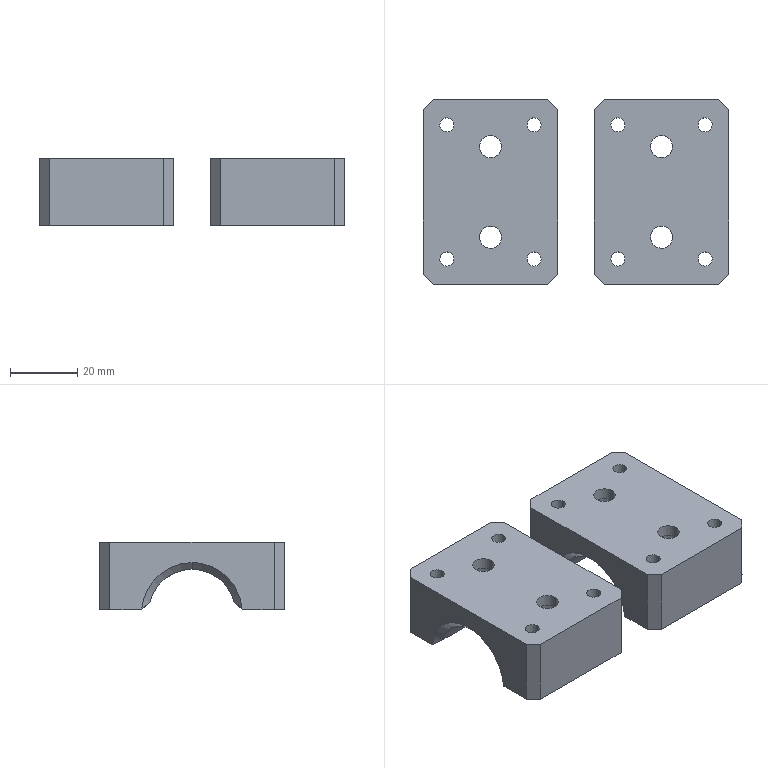NC program | NX | posted with a generic post | part box 91 x 55 x 20 mm
Lines 4306 to 5121 of 95737:
(FIXED_CONTOUR , TOOL : R3)
N8562 T17 M6
N8564 G54
N8566 G17 G0 G90 X3.472 Y-12.781 S9500 M3
N8568 G43 Z30. H17
N8570 Z2.4
N8572 G94 G1 Z-2.825 F1000.
N8574 X3.459 Y-12.768 Z-2.953 F3000.
N8576 X3.448 Y-12.757 Z-3.126
N8578 X3.439 Y-12.747 Z-3.346
N8580 X3.43 Y-12.738 Z-3.478
N8582 X3.419 Y-12.727 Z-3.695
N8584 X3.394 Y-12.702 Z-3.972
N8586 X3.383 Y-12.692 Z-4.138
N8588 X3.386 Y-12.662 Z-4.327
N8590 X3.385 Y-12.623 Z-4.543
N8592 X3.387 Y-12.596 Z-4.676
N8594 Y-12.576 Z-4.761
N8596 X3.397 Y-12.586 Z-4.673
N8598 X3.423 Y-12.613 Z-4.381
N8600 X3.44 Y-12.629 Z-4.127
N8602 X3.474 Y-12.664 Z-3.74
N8604 X3.483 Y-12.673 Z-3.565
N8606 X3.496 Y-12.686 Z-3.375
N8608 X3.504 Y-12.693 Z-3.202
N8610 X3.519 Y-12.708 Z-2.965
N8612 X3.535 Y-12.724 Z-2.813
N8614 X3.546 Y-12.735 Z-2.689
N8616 X3.575 Y-12.72 Z-2.638
N8618 X3.626 Y-12.697 Z-2.555
N8620 X3.609 Y-12.679 Z-2.674
N8622 X3.6 Y-12.671 Z-2.774
N8624 X3.578 Y-12.648 Z-2.991
N8626 X3.559 Y-12.63 Z-3.278
N8628 X3.554 Y-12.624 Z-3.404
N8630 X3.537 Y-12.607 Z-3.652
N8632 X3.53 Y-12.6 Z-3.785
N8634 X3.486 Y-12.556 Z-4.282
N8636 X3.475 Y-12.545 Z-4.455
N8638 X3.457 Y-12.527 Z-4.654
N8640 X3.396 Y-12.466 Z-5.176
N8642 X3.382 Y-12.453 Z-5.272
N8644 X3.381 Y-12.401 Z-5.46
N8646 X3.421 Y-12.441 Z-5.166
N8648 X3.482 Y-12.502 Z-4.646
N8650 X3.496 Y-12.516 Z-4.486
N8652 X3.505 Y-12.525 Z-4.348
N8654 X3.554 Y-12.574 Z-3.804
N8656 X3.56 Y-12.58 Z-3.689
N8658 X3.578 Y-12.598 Z-3.416
N8660 X3.583 Y-12.603 Z-3.31
N8662 X3.604 Y-12.624 Z-2.981
N8664 X3.628 Y-12.648 Z-2.757
N8666 X3.634 Y-12.654 Z-2.683
N8668 X3.661 Y-12.681 Z-2.499
N8670 X3.697 Y-12.667 Z-2.442
N8672 X3.659 Y-12.629 Z-2.693
N8674 X3.629 Y-12.598 Z-2.995
N8676 X3.606 Y-12.576 Z-3.343
N8678 X3.602 Y-12.572 Z-3.428
N8680 X3.582 Y-12.552 Z-3.726
N8682 X3.577 Y-12.547 Z-3.823
N8684 X3.525 Y-12.495 Z-4.413
N8686 X3.518 Y-12.488 Z-4.518
N8688 X3.507 Y-12.477 Z-4.638
N8690 X3.446 Y-12.416 Z-5.157
N8692 X3.379 Y-12.349 Z-5.647
N8694 X3.377 Y-12.297 Z-5.805
N8696 X3.41 Y-12.33 Z-5.607
N8698 X3.471 Y-12.391 Z-5.149
N8700 X3.532 Y-12.452 Z-4.63
N8702 X3.54 Y-12.459 Z-4.549
N8704 X3.544 Y-12.464 Z-4.479
N8706 X3.601 Y-12.52 Z-3.842
N8708 X3.605 Y-12.524 Z-3.763
N8710 X3.627 Y-12.546 Z-3.44
N8712 X3.63 Y-12.549 Z-3.375
N8714 X3.654 Y-12.574 Z-2.991
N8716 X3.685 Y-12.604 Z-2.702
N8718 X3.714 Y-12.633 Z-2.503
N8720 X3.736 Y-12.655 Z-2.387
N8722 X3.777 Y-12.645 Z-2.329
N8724 X3.751 Y-12.618 Z-2.459
N8726 X3.737 Y-12.604 Z-2.543
N8728 X3.711 Y-12.578 Z-2.713
N8730 X3.681 Y-12.548 Z-2.996
N8732 X3.652 Y-12.519 Z-3.453
N8734 X3.625 Y-12.492 Z-3.862
N8736 X3.559 Y-12.426 Z-4.622
N8738 X3.498 Y-12.365 Z-5.144
N8740 X3.437 Y-12.304 Z-5.602
N8742 X3.423 Y-12.29 Z-5.693
N8744 X3.377 Y-12.244 Z-5.964
N8746 Y-12.19 Z-6.129
N8748 X3.389 Y-12.202 Z-6.046
N8750 X3.446 Y-12.259 Z-5.714
N8752 X3.464 Y-12.276 Z-5.597
N8754 X3.525 Y-12.337 Z-5.139
N8756 X3.586 Y-12.398 Z-4.613
N8758 X3.651 Y-12.463 Z-3.883
N8760 X3.708 Y-12.52 Z-3.002
N8762 X3.738 Y-12.551 Z-2.728
N8764 X3.769 Y-12.581 Z-2.53
N8766 X3.777 Y-12.59 Z-2.483
N8768 X3.813 Y-12.625 Z-2.31
N8770 X3.822 Y-12.635 Z-2.269
N8772 X3.87 Y-12.626 Z-2.206
N8774 X3.845 Y-12.601 Z-2.31
N8776 X3.804 Y-12.56 Z-2.509
N8778 X3.784 Y-12.54 Z-2.628
N8780 X3.767 Y-12.523 Z-2.744
N8782 X3.736 Y-12.492 Z-3.012
N8784 X3.677 Y-12.433 Z-3.904
N8786 X3.614 Y-12.37 Z-4.609
N8788 X3.553 Y-12.309 Z-5.134
N8790 X3.492 Y-12.248 Z-5.592
N8792 X3.471 Y-12.226 Z-5.735
N8794 X3.401 Y-12.156 Z-6.144
N8796 X3.378 Y-12.133 Z-6.301
N8798 Y-12.098 Z-6.41
N8800 X3.38 Y-12.073 Z-6.478
N8802 X3.413 Y-12.106 Z-6.252
N8804 X3.498 Y-12.19 Z-5.759
N8806 X3.524 Y-12.217 Z-5.587
N8808 X3.585 Y-12.278 Z-5.128
N8810 X3.646 Y-12.339 Z-4.605
N8812 X3.707 Y-12.4 Z-3.928
N8814 X3.768 Y-12.461 Z-3.023
N8816 X3.78 Y-12.473 Z-2.926
N8818 X3.799 Y-12.491 Z-2.762
N8820 X3.835 Y-12.527 Z-2.537
N8822 X3.881 Y-12.574 Z-2.31
N8824 X3.924 Y-12.616 Z-2.136
N8826 X3.956 Y-12.611 Z-2.096
N8828 X3.987 Y-12.609 Z-2.06
N8830 X3.961 Y-12.583 Z-2.152
N8832 X3.919 Y-12.541 Z-2.326
N8834 X3.864 Y-12.487 Z-2.591
N8836 X3.834 Y-12.456 Z-2.782
N8838 X3.823 Y-12.445 Z-2.883
N8840 X3.803 Y-12.426 Z-3.035
N8842 X3.742 Y-12.365 Z-3.924
N8844 X3.681 Y-12.304 Z-4.6
N8846 X3.62 Y-12.243 Z-5.122
N8848 X3.559 Y-12.182 Z-5.581
N8850 X3.528 Y-12.15 Z-5.786
N8852 X3.427 Y-12.05 Z-6.373
N8854 X3.405 Y-12.027 Z-6.528
N8856 X3.383 Y-12.006 Z-6.656
N8858 X3.384 Y-11.991 Z-6.694
N8860 X3.381 Y-11.934 Z-6.833
N8862 X3.411 Y-11.964 Z-6.684
N8864 X3.428 Y-11.981 Z-6.585
N8866 X3.442 Y-11.994 Z-6.493
N8868 X3.558 Y-12.111 Z-5.813
N8870 X3.594 Y-12.147 Z-5.575
N8872 X3.655 Y-12.208 Z-5.116
N8874 X3.716 Y-12.269 Z-4.595
N8876 X3.777 Y-12.33 Z-3.92
N8878 X3.838 Y-12.391 Z-3.048
N8880 X3.872 Y-12.424 Z-2.782
N8882 X3.902 Y-12.454 Z-2.6
N8884 X3.96 Y-12.513 Z-2.318
N8886 X4.01 Y-12.562 Z-2.125
N8888 X4.054 Y-12.606 Z-1.983
N8890 X4.122 Y-12.605 Z-1.907
N8892 X4.091 Y-12.574 Z-1.999
N8894 X4.042 Y-12.525 Z-2.162
N8896 X3.995 Y-12.478 Z-2.342
N8898 X3.935 Y-12.418 Z-2.631
N8900 X3.899 Y-12.382 Z-2.856
N8902 X3.873 Y-12.356 Z-3.061
N8904 X3.865 Y-12.347 Z-3.165
N8906 X3.812 Y-12.295 Z-3.917
N8908 X3.751 Y-12.234 Z-4.59
N8910 X3.69 Y-12.173 Z-5.11
N8912 X3.629 Y-12.112 Z-5.568
N8914 X3.588 Y-12.071 Z-5.839
N8916 X3.446 Y-11.929 Z-6.671
N8918 X3.38 Y-11.862 Z-7.01
N8920 X3.378 Y-11.784 Z-7.181
N8922 X3.412 Y-11.818 Z-7.032
N8924 X3.485 Y-11.891 Z-6.661
N8926 X3.621 Y-12.027 Z-5.868
N8928 X3.668 Y-12.074 Z-5.562
N8930 X3.736 Y-12.142 Z-5.041
N8932 X3.79 Y-12.196 Z-4.585
N8934 X3.851 Y-12.257 Z-3.912
N8936 X3.895 Y-12.301 Z-3.269
N8938 X3.912 Y-12.318 Z-3.076
N8940 X3.942 Y-12.348 Z-2.842
N8942 X3.973 Y-12.379 Z-2.659
N8944 X4.034 Y-12.44 Z-2.369
N8946 X4.088 Y-12.494 Z-2.162
N8948 X4.142 Y-12.549 Z-1.986
N8950 X4.197 Y-12.603 Z-1.824
N8952 X4.277 Y-12.609 Z-1.743
N8954 X4.252 Y-12.584 Z-1.807
N8956 X4.192 Y-12.524 Z-1.975
N8958 X4.128 Y-12.46 Z-2.181
N8960 X4.071 Y-12.403 Z-2.396
N8962 X4.01 Y-12.342 Z-2.682
N8964 X3.98 Y-12.311 Z-2.862
N8966 X3.949 Y-12.281 Z-3.09
N8968 X3.925 Y-12.257 Z-3.37
N8970 X3.888 Y-12.22 Z-3.908
N8972 X3.827 Y-12.159 Z-4.58
N8974 X3.766 Y-12.098 Z-5.096
N8976 X3.705 Y-12.037 Z-5.555
N8978 X3.652 Y-11.984 Z-5.9
N8980 X3.522 Y-11.854 Z-6.653
N8982 X3.444 Y-11.776 Z-7.049
N8984 X3.388 Y-11.72 Z-7.297
N8986 X3.378 Y-11.71 Z-7.346
N8988 X3.379 Y-11.639 Z-7.504
N8990 X3.403 Y-11.663 Z-7.386
N8992 X3.475 Y-11.735 Z-7.065
N8994 X3.558 Y-11.818 Z-6.645
N8996 X3.684 Y-11.944 Z-5.925
N8998 X3.741 Y-12.001 Z-5.549
N9000 X3.802 Y-12.062 Z-5.09
N9002 X3.863 Y-12.123 Z-4.575
N9004 X3.924 Y-12.184 Z-3.904
N9006 X3.956 Y-12.216 Z-3.448
N9008 X3.985 Y-12.245 Z-3.105
N9010 X4.016 Y-12.276 Z-2.881
N9012 X4.046 Y-12.306 Z-2.704
N9014 X4.107 Y-12.367 Z-2.42
N9016 X4.166 Y-12.426 Z-2.198
N9018 X4.226 Y-12.486 Z-2.007
N9020 X4.306 Y-12.566 Z-1.788
N9022 X4.357 Y-12.617 Z-1.666
N9024 X4.44 Y-12.627 Z-1.588
N9026 X4.398 Y-12.585 Z-1.682
N9028 X4.345 Y-12.532 Z-1.81
N9030 X4.259 Y-12.445 Z-2.047
N9032 X4.205 Y-12.392 Z-2.219
N9034 X4.144 Y-12.331 Z-2.446
N9036 X4.083 Y-12.27 Z-2.726
N9038 X4.052 Y-12.239 Z-2.901
N9040 X4.022 Y-12.209 Z-3.121
N9042 X4.005 Y-12.191 Z-3.321
N9044 X3.991 Y-12.178 Z-3.458
N9046 X3.961 Y-12.148 Z-3.9
N9048 X3.9 Y-12.087 Z-4.57
N9050 X3.839 Y-12.026 Z-5.083
N9052 X3.778 Y-11.965 Z-5.543
N9054 X3.717 Y-11.904 Z-5.942
N9056 X3.595 Y-11.782 Z-6.637
N9058 X3.506 Y-11.693 Z-7.082
N9060 X3.417 Y-11.604 Z-7.478
N9062 X3.382 Y-11.568 Z-7.655
N9064 X3.383 Y-11.493 Z-7.808
N9066 X3.414 Y-11.523 Z-7.672
N9068 X3.433 Y-11.542 Z-7.575
N9070 X3.539 Y-11.649 Z-7.1
N9072 X3.634 Y-11.743 Z-6.629
N9074 X3.756 Y-11.865 Z-5.935
N9076 X3.817 Y-11.926 Z-5.537
N9078 X3.878 Y-11.987 Z-5.076
N9080 X3.939 Y-12.048 Z-4.565
N9082 X4. Y-12.109 Z-3.896
N9084 X4.03 Y-12.14 Z-3.459
N9086 X4.061 Y-12.17 Z-3.137
N9088 X4.097 Y-12.207 Z-2.885
N9090 X4.122 Y-12.231 Z-2.75
N9092 X4.183 Y-12.292 Z-2.472
N9094 X4.244 Y-12.353 Z-2.247
N9096 X4.293 Y-12.403 Z-2.088
N9098 X4.385 Y-12.494 Z-1.837
N9100 X4.467 Y-12.577 Z-1.644
N9102 X4.487 Y-12.597 Z-1.6
N9104 X4.536 Y-12.646 Z-1.505
N9106 X4.638 Y-12.667 Z-1.419
N9108 X4.52 Y-12.549 Z-1.649
N9110 X4.495 Y-12.524 Z-1.705
N9112 X4.415 Y-12.444 Z-1.895
N9114 X4.337 Y-12.366 Z-2.11
N9116 X4.284 Y-12.313 Z-2.276
N9118 X4.223 Y-12.252 Z-2.5
N9120 X4.162 Y-12.191 Z-2.774
N9122 X4.132 Y-12.16 Z-2.944
N9124 X4.101 Y-12.13 Z-3.155
N9126 X4.071 Y-12.099 Z-3.462
N9128 X4.04 Y-12.069 Z-3.892
N9130 X3.979 Y-12.008 Z-4.559
N9132 X3.918 Y-11.947 Z-5.069
N9134 X3.857 Y-11.886 Z-5.53
N9136 X3.796 Y-11.825 Z-5.928
N9138 X3.674 Y-11.703 Z-6.621
N9140 X3.574 Y-11.603 Z-7.118
N9142 X3.449 Y-11.478 Z-7.675
N9144 X3.43 Y-11.459 Z-7.766
N9146 X3.381 Y-11.41 Z-7.967
N9148 Y-11.373 Z-8.039
N9150 Y-11.324 Z-8.124
N9152 X3.402 Y-11.345 Z-8.046
N9154 X3.485 Y-11.428 Z-7.7
N9156 X3.611 Y-11.553 Z-7.14
N9158 X3.717 Y-11.66 Z-6.611
N9160 X3.839 Y-11.782 Z-5.92
N9162 X3.9 Y-11.843 Z-5.522
N9164 X3.961 Y-11.904 Z-5.061
N9166 X4.022 Y-11.965 Z-4.553
N9168 X4.083 Y-12.026 Z-3.887
N9170 X4.114 Y-12.056 Z-3.466
N9172 X4.13 Y-12.073 Z-3.295
N9174 X4.144 Y-12.087 Z-3.175
N9176 X4.175 Y-12.117 Z-2.968
N9178 X4.209 Y-12.151 Z-2.788
N9180 X4.266 Y-12.209 Z-2.529
N9182 X4.327 Y-12.27 Z-2.307
N9184 X4.388 Y-12.331 Z-2.118
N9186 X4.452 Y-12.395 Z-1.944
N9188 X4.56 Y-12.502 Z-1.692
N9190 X4.571 Y-12.514 Z-1.666
N9192 X4.693 Y-12.636 Z-1.43
N9194 X4.733 Y-12.675 Z-1.363
N9196 X4.755 Y-12.697 Z-1.328
N9198 X4.885 Y-12.74 Z-1.236
N9200 X4.814 Y-12.669 Z-1.339
N9202 X4.749 Y-12.604 Z-1.445
N9204 X4.615 Y-12.47 Z-1.701
N9206 X4.493 Y-12.348 Z-1.984
N9208 X4.429 Y-12.285 Z-2.16
N9210 X4.371 Y-12.226 Z-2.339
N9212 X4.31 Y-12.165 Z-2.559
N9214 X4.249 Y-12.104 Z-2.828
N9216 X4.214 Y-12.069 Z-3.02
N9218 X4.188 Y-12.043 Z-3.195
N9220 X4.165 Y-12.021 Z-3.39
N9222 X4.158 Y-12.013 Z-3.47
N9224 X4.127 Y-11.982 Z-3.882
N9226 X4.066 Y-11.921 Z-4.547
N9228 X4.005 Y-11.86 Z-5.055
N9230 X3.944 Y-11.799 Z-5.514
N9232 X3.883 Y-11.738 Z-5.912
N9234 X3.761 Y-11.616 Z-6.602
N9236 X3.649 Y-11.504 Z-7.159
N9238 X3.517 Y-11.372 Z-7.74
N9240 X3.44 Y-11.295 Z-8.058
N9242 X3.382 Y-11.237 Z-8.274
N9244 Y-11.149 Z-8.425
N9246 X3.478 Y-11.244 Z-8.071
N9248 X3.562 Y-11.328 Z-7.729
N9250 X3.691 Y-11.458 Z-7.156
N9252 X3.806 Y-11.572 Z-6.592
N9254 X3.928 Y-11.694 Z-5.904
N9256 X3.989 Y-11.755 Z-5.506
N9258 X4.05 Y-11.816 Z-5.049
N9260 X4.111 Y-11.877 Z-4.541
N9262 X4.172 Y-11.938 Z-3.878
N9264 X4.204 Y-11.971 Z-3.459
N9266 X4.233 Y-11.999 Z-3.215
N9268 X4.25 Y-12.017 Z-3.099
N9270 X4.294 Y-12.06 Z-2.855
N9272 X4.355 Y-12.121 Z-2.589
N9274 X4.416 Y-12.182 Z-2.371
N9276 X4.477 Y-12.243 Z-2.184
N9278 X4.538 Y-12.304 Z-2.018
N9280 X4.57 Y-12.336 Z-1.941
N9282 X4.66 Y-12.426 Z-1.736
N9284 X4.79 Y-12.557 Z-1.486
N9286 X4.865 Y-12.632 Z-1.365
N9288 X5.018 Y-12.785 Z-1.144
N9290 X5.166 Y-12.844 Z-1.05
N9292 X5.07 Y-12.748 Z-1.17
N9294 X4.916 Y-12.594 Z-1.391
N9296 X4.826 Y-12.504 Z-1.538
N9298 X4.704 Y-12.382 Z-1.772
N9300 X4.629 Y-12.307 Z-1.94
N9302 X4.582 Y-12.26 Z-2.052
N9304 X4.521 Y-12.199 Z-2.217
N9306 X4.454 Y-12.131 Z-2.425
N9308 X4.399 Y-12.077 Z-2.619
N9310 X4.338 Y-12.016 Z-2.883
N9312 X4.286 Y-11.963 Z-3.178
N9314 X4.277 Y-11.955 Z-3.234
N9316 X4.247 Y-11.924 Z-3.482
N9318 X4.216 Y-11.894 Z-3.872
N9320 X4.155 Y-11.833 Z-4.535
N9322 X4.094 Y-11.772 Z-5.043
N9324 X4.033 Y-11.711 Z-5.498
N9326 X3.972 Y-11.65 Z-5.896
N9328 X3.85 Y-11.528 Z-6.582
N9330 X3.728 Y-11.406 Z-7.183
N9332 X3.606 Y-11.284 Z-7.717
N9334 X3.516 Y-11.194 Z-8.083
N9336 X3.383 Y-11.06 Z-8.578
N9338 Y-10.986 Z-8.707
N9340 X3.548 Y-11.151 Z-8.094
N9342 X3.644 Y-11.246 Z-7.708
N9344 X3.766 Y-11.368 Z-7.174
N9346 X3.888 Y-11.49 Z-6.574
N9348 X4.01 Y-11.612 Z-5.889
N9350 X4.071 Y-11.673 Z-5.491
N9352 X4.132 Y-11.734 Z-5.037
N9354 X4.193 Y-11.795 Z-4.53
N9356 X4.254 Y-11.856 Z-3.867
N9358 X4.285 Y-11.887 Z-3.492
N9360 X4.316 Y-11.918 Z-3.245
N9362 X4.376 Y-11.978 Z-2.906
N9364 X4.437 Y-12.039 Z-2.645
N9366 X4.498 Y-12.1 Z-2.43
N9368 X4.559 Y-12.161 Z-2.245
N9370 X4.62 Y-12.222 Z-2.081
N9372 X4.686 Y-12.288 Z-1.924
N9374 X4.742 Y-12.344 Z-1.801
N9376 X4.872 Y-12.474 Z-1.555
N9378 X4.959 Y-12.561 Z-1.413
N9380 X5.108 Y-12.71 Z-1.2
N9382 X5.176 Y-12.778 Z-1.114
N9384 X5.23 Y-12.832 Z-1.051
N9386 X5.31 Y-12.912 Z-0.969
N9388 X4.758 Y-12.36 Z3.767
N9390 G0 X4.92 Y-13.022
N9392 G1 Z-0.73 F1000.
N9394 G2 X5.5 Y-13.177 R0.6
N9396 G1 X5.508 Y-13.185 Z-0.724 F3000.
N9398 X5.583
N9400 X5.498 Y-13.101 Z-0.794
N9402 G3 X4.919 Y-12.945 R0.6
N9404 G1 Z3.026
N9406 G0 X5.062 Y-12.886
N9408 G1 Z-0.724 F1000.
N9410 G3 X5.583 Y-13.185 R0.6
N9412 G1 X5.673 Z-0.723 F3000.
N9414 X5.618 Y-13.13 Z-0.768
N9416 X5.52 Y-13.031 Z-0.853
N9418 X5.386 Y-12.897 Z-0.975
N9420 X5.263 Y-12.775 Z-1.104
N9422 X5.176 Y-12.687 Z-1.209
N9424 X5.154 Y-12.665 Z-1.237
N9426 X5.011 Y-12.523 Z-1.44
N9428 X4.91 Y-12.421 Z-1.605
N9430 X4.788 Y-12.299 Z-1.837
N9432 X4.719 Y-12.23 Z-1.989
N9434 X4.659 Y-12.17 Z-2.134
N9436 X4.605 Y-12.116 Z-2.278
N9438 X4.544 Y-12.055 Z-2.463
N9440 X4.483 Y-11.994 Z-2.676
N9442 X4.419 Y-11.93 Z-2.95
N9444 X4.361 Y-11.872 Z-3.27
N9446 X4.33 Y-11.842 Z-3.504
N9448 X4.32 Y-11.831 Z-3.606
N9450 X4.3 Y-11.811 Z-3.862
N9452 X4.239 Y-11.75 Z-4.523
N9454 X4.178 Y-11.689 Z-5.031
N9456 X4.117 Y-11.628 Z-5.483
N9458 X4.056 Y-11.567 Z-5.88
N9460 X3.934 Y-11.445 Z-6.564
N9462 X3.812 Y-11.323 Z-7.163
N9464 X3.69 Y-11.201 Z-7.696
N9466 X3.588 Y-11.099 Z-8.107
N9468 X3.43 Y-10.941 Z-8.694
N9470 X3.382 Y-10.894 Z-8.863
N9472 X3.383 Y-10.799 Z-9.004
N9474 X3.419 Y-10.835 Z-8.885
N9476 X3.494 Y-10.91 Z-8.624
N9478 X3.629 Y-11.045 Z-8.121
N9480 X3.738 Y-11.154 Z-7.684
N9482 X3.86 Y-11.276 Z-7.151
N9484 X3.982 Y-11.398 Z-6.554
N9486 X4.104 Y-11.52 Z-5.872
N9488 X4.171 Y-11.587 Z-5.427
N9490 X4.226 Y-11.642 Z-5.024
N9492 X4.287 Y-11.703 Z-4.517
N9494 X4.348 Y-11.764 Z-3.855
N9496 X4.361 Y-11.777 Z-3.686
N9498 X4.378 Y-11.794 Z-3.517
N9500 X4.409 Y-11.825 Z-3.291
N9502 X4.47 Y-11.886 Z-2.963
N9504 X4.531 Y-11.947 Z-2.709
N9506 X4.592 Y-12.008 Z-2.497
N9508 X4.653 Y-12.069 Z-2.314
N9510 X4.714 Y-12.13 Z-2.152
N9512 X4.757 Y-12.173 Z-2.048
N9514 X4.836 Y-12.252 Z-1.875
N9516 X4.958 Y-12.374 Z-1.644
N9518 X5.066 Y-12.482 Z-1.468
N9520 X5.202 Y-12.618 Z-1.276
N9522 X5.301 Y-12.717 Z-1.155
N9524 X5.428 Y-12.844 Z-1.02
N9526 X5.446 Y-12.862 Z-1.002
N9528 X5.568 Y-12.984 Z-0.893
N9530 X5.714 Y-13.13 Z-0.768
N9532 X5.769 Y-13.185 Z-0.723
N9534 X5.865
N9536 X5.81 Y-13.13 Z-0.768
N9538 X5.616 Y-12.936 Z-0.934
N9540 X5.489 Y-12.809 Z-1.048
N9542 X5.352 Y-12.672 Z-1.192
N9544 X5.25 Y-12.57 Z-1.316
N9546 X5.121 Y-12.441 Z-1.497
N9548 X5.006 Y-12.326 Z-1.682
N9550 X4.884 Y-12.204 Z-1.913
N9552 X4.796 Y-12.115 Z-2.108
N9554 X4.762 Y-12.082 Z-2.189
N9556 X4.701 Y-12.021 Z-2.349
N9558 X4.64 Y-11.96 Z-2.532
N9560 X4.574 Y-11.894 Z-2.762
N9562 X4.518 Y-11.838 Z-2.992
N9564 X4.503 Y-11.822 Z-3.066
N9566 X4.455 Y-11.775 Z-3.323
N9568 X4.426 Y-11.746 Z-3.53
N9570 X4.402 Y-11.722 Z-3.767
N9572 X4.396 Y-11.716 Z-3.849
N9574 X4.335 Y-11.655 Z-4.51
N9576 X4.274 Y-11.594 Z-5.018
N9578 X4.213 Y-11.533 Z-5.466
N9580 X4.152 Y-11.472 Z-5.863
N9582 X4.03 Y-11.35 Z-6.543
N9584 X3.908 Y-11.228 Z-7.139
N9586 X3.786 Y-11.106 Z-7.672
N9588 X3.67 Y-10.99 Z-8.134
N9590 X3.542 Y-10.862 Z-8.61
N9592 X3.461 Y-10.781 Z-8.893
N9594 X3.383 Y-10.703 Z-9.146
N9596 Y-10.606 Z-9.289
N9598 X3.503 Y-10.725 Z-8.901
N9600 X3.591 Y-10.813 Z-8.596
N9602 X3.713 Y-10.935 Z-8.145
N9604 X3.835 Y-11.057 Z-7.659
N9606 X3.957 Y-11.179 Z-7.127
N9608 X4.079 Y-11.301 Z-6.532
N9610 X4.201 Y-11.423 Z-5.854
N9612 X4.262 Y-11.484 Z-5.457
N9614 X4.323 Y-11.545 Z-5.012
N9616 X4.384 Y-11.606 Z-4.504
N9618 X4.443 Y-11.666 Z-3.855
N9620 X4.471 Y-11.694 Z-3.573
N9622 X4.498 Y-11.721 Z-3.378
N9624 X4.542 Y-11.764 Z-3.142
N9626 X4.567 Y-11.789 Z-3.02
N9628 X4.628 Y-11.85 Z-2.773
N9630 X4.688 Y-11.911 Z-2.568
N9632 X4.75 Y-11.972 Z-2.386
N9634 X4.811 Y-12.033 Z-2.226
N9636 X4.835 Y-12.057 Z-2.168
N9638 X4.933 Y-12.155 Z-1.951
N9640 X5.055 Y-12.277 Z-1.721
N9642 X5.176 Y-12.399 Z-1.526
N9644 X5.299 Y-12.521 Z-1.357
N9646 X5.421 Y-12.643 Z-1.211
N9648 X5.543 Y-12.765 Z-1.085
N9650 X5.664 Y-12.887 Z-0.976
N9652 X5.907 Y-13.13 Z-0.768
N9654 X5.962 Y-13.185 Z-0.723
N9656 X6.06
N9658 X6.005 Y-13.13 Z-0.768
N9660 X5.698 Y-12.822 Z-1.031
N9662 X5.592 Y-12.716 Z-1.126
N9664 X5.464 Y-12.588 Z-1.259
N9666 X5.348 Y-12.472 Z-1.398
N9668 X5.226 Y-12.35 Z-1.566
N9670 X5.104 Y-12.228 Z-1.761
N9672 X4.982 Y-12.106 Z-1.989
N9674 X4.86 Y-11.984 Z-2.263
N9676 X4.799 Y-11.923 Z-2.422
N9678 X4.728 Y-11.852 Z-2.634
N9680 X4.677 Y-11.801 Z-2.805
N9682 X4.616 Y-11.74 Z-3.049
N9684 X4.581 Y-11.706 Z-3.219
N9686 X4.542 Y-11.667 Z-3.434
N9688 X4.515 Y-11.64 Z-3.63
N9690 X4.476 Y-11.601 Z-4.026
N9692 X4.433 Y-11.557 Z-4.497
N9694 X4.372 Y-11.496 Z-5.006
N9696 X4.311 Y-11.435 Z-5.447
N9698 X4.25 Y-11.374 Z-5.845
N9700 X4.128 Y-11.252 Z-6.522
N9702 X4.006 Y-11.13 Z-7.115
N9704 X3.884 Y-11.008 Z-7.647
N9706 X3.762 Y-10.886 Z-8.13
N9708 X3.64 Y-10.764 Z-8.581
N9710 X3.545 Y-10.669 Z-8.91
N9712 X3.383 Y-10.508 Z-9.434
N9714 X3.382 Y-10.408 Z-9.579
N9716 X3.455 Y-10.481 Z-9.349
N9718 X3.587 Y-10.613 Z-8.918
N9720 X3.689 Y-10.715 Z-8.567
N9722 X3.811 Y-10.837 Z-8.116
N9724 X3.933 Y-10.959 Z-7.634
N9726 X4.055 Y-11.081 Z-7.103
N9728 X4.177 Y-11.203 Z-6.511
N9730 X4.299 Y-11.325 Z-5.836
N9732 X4.36 Y-11.386 Z-5.438
N9734 X4.421 Y-11.447 Z-4.999
N9736 X4.482 Y-11.508 Z-4.49
N9738 X4.543 Y-11.569 Z-3.846
N9740 X4.559 Y-11.585 Z-3.686
N9742 X4.586 Y-11.612 Z-3.49
N9744 X4.621 Y-11.646 Z-3.296
N9746 X4.665 Y-11.691 Z-3.078
N9748 X4.726 Y-11.752 Z-2.838
N9750 X4.787 Y-11.813 Z-2.635
N9752 X4.848 Y-11.874 Z-2.458
N9754 X4.914 Y-11.939 Z-2.29
N9756 X5.031 Y-12.057 Z-2.028
N9758 X5.153 Y-12.179 Z-1.801
N9760 X5.275 Y-12.301 Z-1.606
N9762 X5.402 Y-12.428 Z-1.433
N9764 X5.519 Y-12.545 Z-1.294
N9766 X5.641 Y-12.667 Z-1.169
N9768 X5.763 Y-12.789 Z-1.059
N9770 X6.104 Y-13.13 Z-0.768
N9772 X6.159 Y-13.185 Z-0.723
N9774 X6.262
N9776 X6.207 Y-13.13 Z-0.768
N9778 X5.765 Y-12.688 Z-1.147
N9780 X5.693 Y-12.616 Z-1.212
N9782 X5.565 Y-12.488 Z-1.344
N9784 X5.44 Y-12.363 Z-1.494
N9786 X5.327 Y-12.25 Z-1.648
N9788 X5.205 Y-12.128 Z-1.842
N9790 X5.083 Y-12.006 Z-2.069
N9792 X4.955 Y-11.878 Z-2.354
N9794 X4.9 Y-11.823 Z-2.496
N9796 X4.839 Y-11.762 Z-2.671
N9798 X4.778 Y-11.701 Z-2.872
N9800 X4.717 Y-11.64 Z-3.109
N9802 X4.656 Y-11.579 Z-3.409
N9804 X4.632 Y-11.555 Z-3.548
N9806 X4.605 Y-11.528 Z-3.746
N9808 X4.534 Y-11.457 Z-4.483
N9810 X4.473 Y-11.396 Z-4.993
N9812 X4.412 Y-11.335 Z-5.429
N9814 X4.351 Y-11.274 Z-5.827
N9816 X4.229 Y-11.152 Z-6.5
N9818 X4.107 Y-11.03 Z-7.091
N9820 X3.985 Y-10.908 Z-7.621
N9822 X3.863 Y-10.786 Z-8.101
N9824 X3.741 Y-10.664 Z-8.552
N9826 X3.631 Y-10.554 Z-8.927
N9828 X3.485 Y-10.408 Z-9.399
N9830 X3.422 Y-10.345 Z-9.596
N9832 X3.383 Y-10.306 Z-9.712
N9834 X3.384 Y-10.203 Z-9.846
N9836 X3.399 Y-10.218 Z-9.799
N9838 X3.467 Y-10.286 Z-9.601
N9840 X3.636 Y-10.455 Z-9.066
N9842 X3.683 Y-10.502 Z-8.912
N9844 X3.793 Y-10.612 Z-8.536
N9846 X3.915 Y-10.734 Z-8.086
N9848 X4.037 Y-10.856 Z-7.608
N9850 X4.159 Y-10.978 Z-7.078
N9852 X4.281 Y-11.1 Z-6.488
N9854 X4.403 Y-11.222 Z-5.817
N9856 X4.464 Y-11.283 Z-5.419
N9858 X4.525 Y-11.344 Z-4.985
N9860 X4.586 Y-11.405 Z-4.476
N9862 X4.652 Y-11.47 Z-3.805
N9864 X4.679 Y-11.498 Z-3.607
N9866 X4.708 Y-11.527 Z-3.433
N9868 X4.769 Y-11.588 Z-3.14
N9870 X4.83 Y-11.649 Z-2.906
N9872 X4.891 Y-11.71 Z-2.707
N9874 X4.952 Y-11.771 Z-2.533
N9876 X5.013 Y-11.832 Z-2.378
N9878 X5.135 Y-11.954 Z-2.11
N9880 X5.257 Y-12.076 Z-1.884
N9882 X5.379 Y-12.198 Z-1.691
N9884 X5.501 Y-12.32 Z-1.525
N9886 X5.636 Y-12.455 Z-1.367
N9888 X5.745 Y-12.564 Z-1.256
N9890 X5.867 Y-12.686 Z-1.148
N9892 X6.311 Y-13.13 Z-0.768
N9894 X6.366 Y-13.185 Z-0.723
N9896 X6.471
N9898 X6.416 Y-13.13 Z-0.768
N9900 X5.92 Y-12.634 Z-1.193
N9902 X5.798 Y-12.512 Z-1.301
N9904 X5.676 Y-12.39 Z-1.425
N9906 X5.554 Y-12.268 Z-1.568
N9908 X5.432 Y-12.146 Z-1.734
N9910 X5.31 Y-12.024 Z-1.926
N9912 X5.184 Y-11.898 Z-2.16
N9914 X5.066 Y-11.78 Z-2.417
N9916 X4.99 Y-11.704 Z-2.611
N9918 X4.944 Y-11.658 Z-2.744
N9920 X4.883 Y-11.597 Z-2.941
N9922 X4.822 Y-11.536 Z-3.171
N9924 X4.786 Y-11.5 Z-3.346
N9926 X4.761 Y-11.475 Z-3.457
N9928 X4.731 Y-11.444 Z-3.632
N9930 X4.698 Y-11.412 Z-3.865
N9932 X4.639 Y-11.353 Z-4.469
N9934 X4.578 Y-11.292 Z-4.978
N9936 X4.517 Y-11.231 Z-5.409
N9938 X4.456 Y-11.17 Z-5.807
N9940 X4.334 Y-11.048 Z-6.477
N9942 X4.212 Y-10.926 Z-7.065
N9944 X4.09 Y-10.804 Z-7.594
N9946 X3.968 Y-10.682 Z-8.071
N9948 X3.846 Y-10.56 Z-8.521
N9950 X3.724 Y-10.438 Z-8.936
N9952 X3.512 Y-10.226 Z-9.605
N9954 X3.42 Y-10.134 Z-9.874
N9956 X3.386 Y-10.1 Z-9.982
N9958 X3.385 Y-9.994 Z-10.117
N9960 X3.428 Y-10.036 Z-9.992
N9962 X3.441 Y-10.05 Z-9.948
N9964 X3.557 Y-10.166 Z-9.609
N9966 X3.777 Y-10.386 Z-8.919
N9968 X3.899 Y-10.508 Z-8.505
N9970 X4.021 Y-10.63 Z-8.056
N9972 X4.143 Y-10.752 Z-7.581
N9974 X4.265 Y-10.874 Z-7.052
N9976 X4.387 Y-10.996 Z-6.465
N9978 X4.509 Y-11.118 Z-5.798
N9980 X4.57 Y-11.179 Z-5.399
N9982 X4.631 Y-11.24 Z-4.971
N9984 X4.692 Y-11.301 Z-4.461
N9986 X4.745 Y-11.354 Z-3.921
N9988 X4.778 Y-11.387 Z-3.684
N9990 X4.814 Y-11.423 Z-3.481
N9992 X4.856 Y-11.465 Z-3.293
N9994 X4.875 Y-11.484 Z-3.202
N9996 X4.936 Y-11.545 Z-2.975
N9998 X4.997 Y-11.606 Z-2.78
N10000 X5.058 Y-11.667 Z-2.609
N10002 X5.119 Y-11.728 Z-2.456
N10004 X5.241 Y-11.85 Z-2.192
N10006 X5.363 Y-11.972 Z-1.968
N10008 X5.485 Y-12.094 Z-1.777
N10010 X5.607 Y-12.216 Z-1.612
N10012 X5.729 Y-12.338 Z-1.469
N10014 X5.851 Y-12.46 Z-1.345
N10016 X5.973 Y-12.582 Z-1.237
N10018 X6.521 Y-13.13 Z-0.768
N10020 X6.576 Y-13.185 Z-0.723
N10022 X6.679
N10024 X6.624 Y-13.13 Z-0.768
N10026 X6.024 Y-12.53 Z-1.281
N10028 X5.902 Y-12.408 Z-1.389
N10030 X5.78 Y-12.286 Z-1.512
N10032 X5.658 Y-12.164 Z-1.655
N10034 X5.536 Y-12.042 Z-1.819
N10036 X5.408 Y-11.914 Z-2.021
N10038 X5.292 Y-11.798 Z-2.231
N10040 X5.254 Y-11.76 Z-2.312
N10042 X5.17 Y-11.676 Z-2.494
N10044 X5.109 Y-11.615 Z-2.646
N10046 X5.048 Y-11.554 Z-2.816
N10048 X4.987 Y-11.493 Z-3.009
N10050 X4.925 Y-11.431 Z-3.24
N10052 X4.865 Y-11.371 Z-3.505
N10054 X4.822 Y-11.328 Z-3.749
N10056 X4.791 Y-11.297 Z-3.976
N10058 X4.743 Y-11.249 Z-4.453
N10060 X4.682 Y-11.188 Z-4.964
N10062 X4.621 Y-11.127 Z-5.39
N10064 X4.56 Y-11.066 Z-5.788
N10066 X4.438 Y-10.944 Z-6.454
N10068 X4.316 Y-10.822 Z-7.039
N10070 X4.194 Y-10.7 Z-7.57
N10072 X4.072 Y-10.578 Z-8.041
N10074 X3.95 Y-10.456 Z-8.49
N10076 X3.828 Y-10.334 Z-8.903
N10078 X3.602 Y-10.108 Z-9.613
N10080 X3.462 Y-9.968 Z-10.022
N10082 X3.383 Y-9.889 Z-10.244
N10084 X3.384 Y-9.785 Z-10.365
N10086 X3.462 Y-9.862 Z-10.145
N10088 X3.497 Y-9.898 Z-10.05
N10090 X3.647 Y-10.048 Z-9.618
N10092 X3.881 Y-10.282 Z-8.885
N10094 X4.003 Y-10.404 Z-8.475
N10096 X4.125 Y-10.526 Z-8.026
N10098 X4.247 Y-10.648 Z-7.554
N10100 X4.369 Y-10.77 Z-7.026
N10102 X4.491 Y-10.892 Z-6.442
N10104 X4.613 Y-11.014 Z-5.779
N10106 X4.674 Y-11.075 Z-5.38
N10108 X4.735 Y-11.136 Z-4.955
N10110 X4.796 Y-11.197 Z-4.445
N10112 X4.838 Y-11.239 Z-4.032
N10114 X4.868 Y-11.268 Z-3.816
N10116 X4.918 Y-11.319 Z-3.53
N10118 X4.979 Y-11.38 Z-3.264
N10120 X5.04 Y-11.441 Z-3.043
N10122 X5.101 Y-11.502 Z-2.852
N10124 X5.165 Y-11.565 Z-2.678
N10126 X5.223 Y-11.624 Z-2.533
N10128 X5.289 Y-11.689 Z-2.39
N10130 X5.345 Y-11.746 Z-2.272
N10132 X5.467 Y-11.868 Z-2.052
N10134 X5.589 Y-11.99 Z-1.862
N10136 X5.711 Y-12.112 Z-1.698
N10138 X5.833 Y-12.234 Z-1.556
N10140 X5.955 Y-12.356 Z-1.434
N10142 X6.077 Y-12.478 Z-1.326
N10144 X6.729 Y-13.13 Z-0.768
N10146 X6.784 Y-13.185 Z-0.723
N10148 X6.892
N10150 X6.837 Y-13.13 Z-0.768
N10152 X6.131 Y-12.424 Z-1.372
N10154 X6.009 Y-12.302 Z-1.479
N10156 X5.887 Y-12.18 Z-1.602
N10158 X5.765 Y-12.058 Z-1.743
N10160 X5.643 Y-11.936 Z-1.906
N10162 X5.521 Y-11.814 Z-2.095
N10164 X5.399 Y-11.692 Z-2.314
N10166 X5.325 Y-11.618 Z-2.469
N10168 X5.277 Y-11.57 Z-2.574
N10170 X5.216 Y-11.509 Z-2.723
N10172 X5.155 Y-11.448 Z-2.89
N10174 X5.094 Y-11.387 Z-3.078
N10176 X5.033 Y-11.326 Z-3.295
N10178 X5.013 Y-11.305 Z-3.377
N10180 X4.964 Y-11.257 Z-3.597
N10182 X4.911 Y-11.204 Z-3.904
N10184 X4.886 Y-11.179 Z-4.09
N10186 X4.85 Y-11.143 Z-4.437